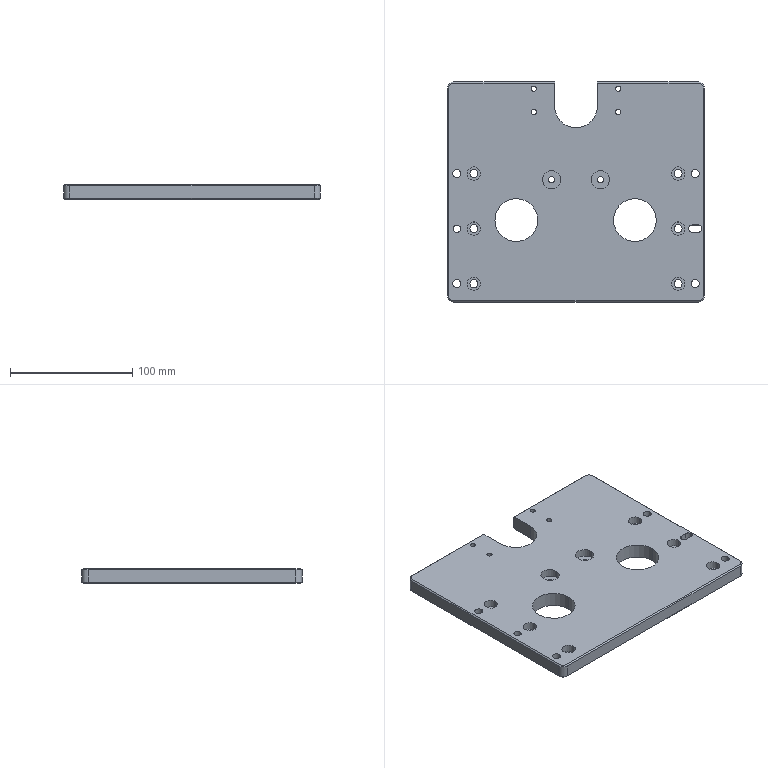Part | STEP file | 06-01-06 support bracket | 1 solid | 99 faces | box 210 x 180 x 12 mm | volume 404728 mm3 | cylinder 62 | plane 29 | cone 8 | commonest cylinder face diameters 6.6 x12 11 x12 4.2 x8 6.5 x8 6 x5 35 x5